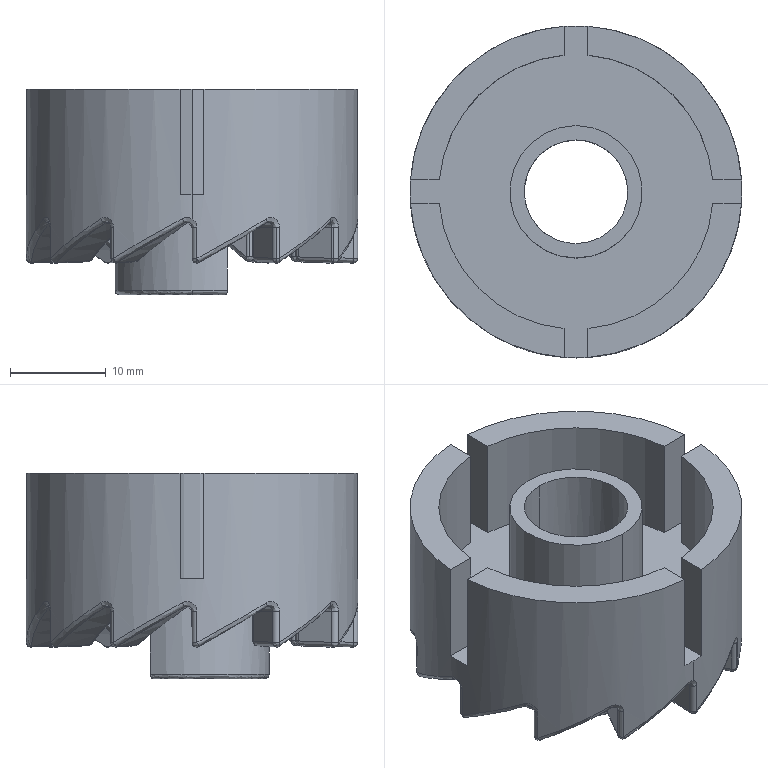Part | SolidWorks | features BaseBody 1 | 1 solid | 199 faces | box 34.702 x 34.702 x 21.496 mm | volume 7230 mm3 | spline 127 | cylinder 42 | plane 30 | commonest cylinder face diameters 1.003 x29 28.684 x4 10.832 x2 13.841 x2 24.672 x2 34.702 x2